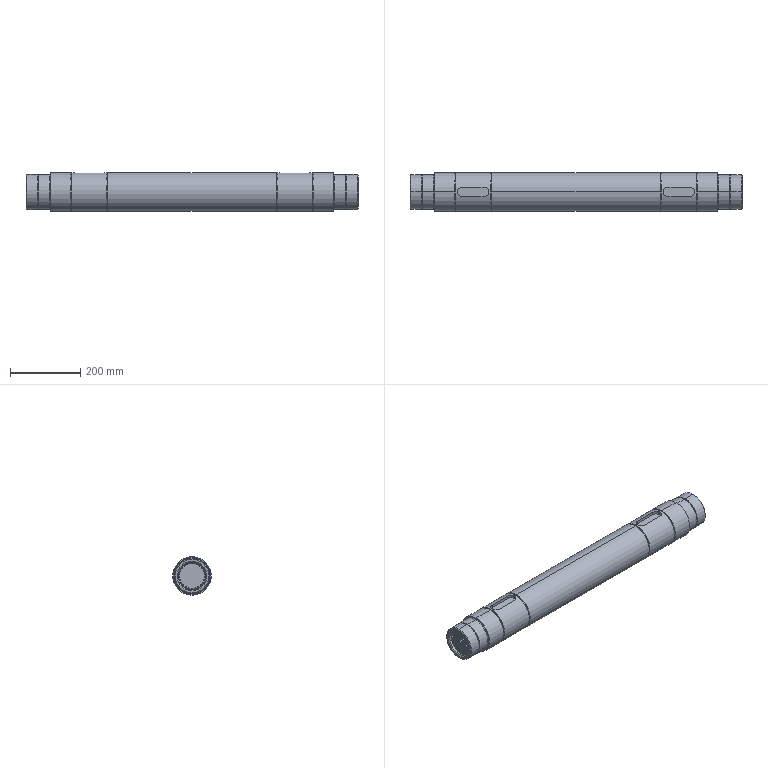Part | SolidWorks | features Chamfer 2, ICE 2, Fillet 1, MirrorSolid 1, Revolution 1 | 1 solid | 552 faces | box 948 x 110 x 110 mm | volume 7904078 mm3 | cylinder 414 | plane 76 | cone 58 | torus 4 | commonest cylinder face diameters 1.2 x120 32.073 x100 38.587 x100 70.8 x50 110 x10 100 x8